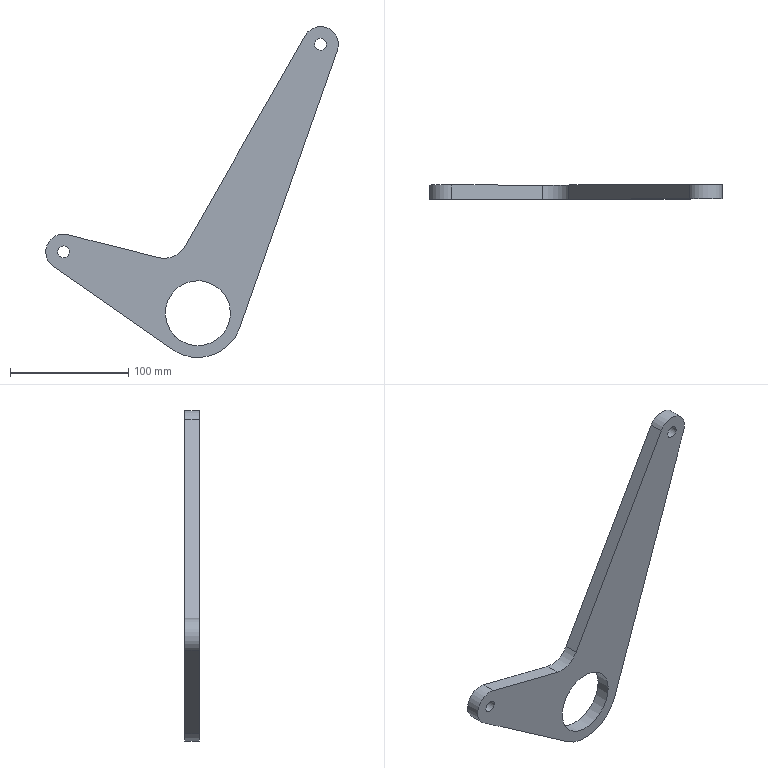Part | NX | features 0 2 | 1 solid | 13 faces | box 247.496 x 12 x 279.945 mm | volume 214925 mm3 | cylinder 7 | plane 6 | commonest cylinder face diameters 10 x2 30 x2 40 x1 55 x1 75 x1
STEP:
#1=CARTESIAN_POINT('',(108.322,86.,-42.76));
#2=VERTEX_POINT('',#1);
#3=CARTESIAN_POINT('',(103.773,86.,-40.685));
#4=DIRECTION('',(0.,-1.,0.));
#5=DIRECTION('',(0.9098,0.,-0.4151));
#6=AXIS2_PLACEMENT_3D('',#3,#4,#5);
#7=CIRCLE('',#6,5.);
#8=EDGE_CURVE('',#2,#2,#7,.T.);
#9=ORIENTED_EDGE('',*,*,#8,.F.);
#10=EDGE_LOOP('',(#9));
#11=FACE_BOUND('',#10,.T.);
#12=CARTESIAN_POINT('',(99.225,74.,-38.609));
#13=VERTEX_POINT('',#12);
#14=CARTESIAN_POINT('',(103.773,74.,-40.685));
#15=DIRECTION('',(0.,1.,0.));
#16=DIRECTION('',(-0.9098,0.,0.4151));
#17=AXIS2_PLACEMENT_3D('',#14,#15,#16);
#18=CIRCLE('',#17,5.);
#19=EDGE_CURVE('',#13,#13,#18,.T.);
#20=ORIENTED_EDGE('',*,*,#19,.F.);
#21=EDGE_LOOP('',(#20));
#22=FACE_BOUND('',#21,.T.);
#23=CARTESIAN_POINT('',(103.773,74.,-40.685));
#24=DIRECTION('',(0.,1.,0.));
#25=DIRECTION('',(-0.9098,0.,0.4151));
#26=AXIS2_PLACEMENT_3D('',#23,#24,#25);
#27=CYLINDRICAL_SURFACE('',#26,5.);
#28=ADVANCED_FACE('',(#11,#22),#27,.F.);
#29=CARTESIAN_POINT('',(-109.173,86.,-218.318));
#30=VERTEX_POINT('',#29);
#31=CARTESIAN_POINT('',(-113.722,86.,-216.243));
#32=DIRECTION('',(0.,-1.,0.));
#33=DIRECTION('',(0.9098,0.,-0.4151));
#34=AXIS2_PLACEMENT_3D('',#31,#32,#33);
#35=CIRCLE('',#34,5.);
#36=EDGE_CURVE('',#30,#30,#35,.T.);
#37=ORIENTED_EDGE('',*,*,#36,.F.);
#38=EDGE_LOOP('',(#37));
#39=FACE_BOUND('',#38,.T.);
#40=CARTESIAN_POINT('',(-118.271,74.,-214.167));
#41=VERTEX_POINT('',#40);
#42=CARTESIAN_POINT('',(-113.722,74.,-216.243));
#43=DIRECTION('',(0.,1.,0.));
#44=DIRECTION('',(-0.9098,0.,0.4151));
#45=AXIS2_PLACEMENT_3D('',#42,#43,#44);
#46=CIRCLE('',#45,5.);
#47=EDGE_CURVE('',#41,#41,#46,.T.);
#48=ORIENTED_EDGE('',*,*,#47,.F.);
#49=EDGE_LOOP('',(#48));
#50=FACE_BOUND('',#49,.T.);
#51=CARTESIAN_POINT('',(-113.722,74.,-216.243));
#52=DIRECTION('',(0.,1.,0.));
#53=DIRECTION('',(-0.9098,0.,0.4151));
#54=AXIS2_PLACEMENT_3D('',#51,#52,#53);
#55=CYLINDRICAL_SURFACE('',#54,5.);
#56=ADVANCED_FACE('',(#39,#50),#55,.F.);
#57=CARTESIAN_POINT('',(35.379,86.,-280.562));
#58=VERTEX_POINT('',#57);
#59=CARTESIAN_POINT('',(35.379,74.,-280.562));
#60=VERTEX_POINT('',#59);
#61=CARTESIAN_POINT('',(35.379,86.,-280.562));
#62=DIRECTION('',(0.,-1.,0.));
#63=VECTOR('',#62,1000.);
#64=LINE('',#61,#63);
#65=EDGE_CURVE('',#58,#60,#64,.T.);
#66=ORIENTED_EDGE('',*,*,#65,.F.);
#67=CARTESIAN_POINT('',(117.925,86.,-45.658));
#68=VERTEX_POINT('',#67);
#69=CARTESIAN_POINT('',(117.925,86.,-45.658));
#70=DIRECTION('',(-0.3315,0.,-0.9434));
#71=VECTOR('',#70,1000.);
#72=LINE('',#69,#71);
#73=EDGE_CURVE('',#68,#58,#72,.T.);
#74=ORIENTED_EDGE('',*,*,#73,.F.);
#75=CARTESIAN_POINT('',(117.925,74.,-45.658));
#76=VERTEX_POINT('',#75);
#77=CARTESIAN_POINT('',(117.925,74.,-45.658));
#78=DIRECTION('',(0.,1.,0.));
#79=VECTOR('',#78,1000.);
#80=LINE('',#77,#79);
#81=EDGE_CURVE('',#76,#68,#80,.T.);
#82=ORIENTED_EDGE('',*,*,#81,.F.);
#83=CARTESIAN_POINT('',(35.379,74.,-280.562));
#84=DIRECTION('',(0.3315,0.,0.9434));
#85=VECTOR('',#84,1000.);
#86=LINE('',#83,#85);
#87=EDGE_CURVE('',#60,#76,#86,.T.);
#88=ORIENTED_EDGE('',*,*,#87,.F.);
#89=EDGE_LOOP('',(#66,#74,#82,#88));
#90=FACE_BOUND('',#89,.T.);
#91=CARTESIAN_POINT('',(117.925,86.,-45.658));
#92=DIRECTION('',(-0.9434,0.,0.3315));
#93=DIRECTION('',(0.3315,0.,0.9434));
#94=AXIS2_PLACEMENT_3D('',#91,#92,#93);
#95=PLANE('',#94);
#96=ADVANCED_FACE('',(#90),#95,.F.);
#97=CARTESIAN_POINT('',(-21.453,86.,-298.887));
#98=VERTEX_POINT('',#97);
#99=CARTESIAN_POINT('',(0.,86.,-268.129));
#100=DIRECTION('',(0.,1.,0.));
#101=DIRECTION('',(0.9098,0.,-0.4151));
#102=AXIS2_PLACEMENT_3D('',#99,#100,#101);
#103=CIRCLE('',#102,37.5);
#104=EDGE_CURVE('',#58,#98,#103,.T.);
#105=ORIENTED_EDGE('',*,*,#104,.F.);
#106=ORIENTED_EDGE('',*,*,#65,.T.);
#107=CARTESIAN_POINT('',(-21.453,74.,-298.887));
#108=VERTEX_POINT('',#107);
#109=CARTESIAN_POINT('',(0.,74.,-268.129));
#110=DIRECTION('',(0.,-1.,0.));
#111=DIRECTION('',(0.9098,0.,-0.4151));
#112=AXIS2_PLACEMENT_3D('',#109,#110,#111);
#113=CIRCLE('',#112,37.5);
#114=EDGE_CURVE('',#108,#60,#113,.T.);
#115=ORIENTED_EDGE('',*,*,#114,.F.);
#116=CARTESIAN_POINT('',(-21.453,74.,-298.887));
#117=DIRECTION('',(0.,1.,0.));
#118=VECTOR('',#117,1000.);
#119=LINE('',#116,#118);
#120=EDGE_CURVE('',#108,#98,#119,.T.);
#121=ORIENTED_EDGE('',*,*,#120,.T.);
#122=EDGE_LOOP('',(#105,#106,#115,#121));
#123=FACE_BOUND('',#122,.T.);
#124=CARTESIAN_POINT('',(0.,86.,-268.129));
#125=DIRECTION('',(0.,-1.,0.));
#126=DIRECTION('',(0.9098,0.,-0.4151));
#127=AXIS2_PLACEMENT_3D('',#124,#125,#126);
#128=CYLINDRICAL_SURFACE('',#127,37.5);
#129=ADVANCED_FACE('',(#123),#128,.T.);
#130=CARTESIAN_POINT('',(-122.303,86.,-228.546));
#131=VERTEX_POINT('',#130);
#132=CARTESIAN_POINT('',(-122.303,74.,-228.546));
#133=VERTEX_POINT('',#132);
#134=CARTESIAN_POINT('',(-122.303,86.,-228.546));
#135=DIRECTION('',(0.,-1.,0.));
#136=VECTOR('',#135,1000.);
#137=LINE('',#134,#136);
#138=EDGE_CURVE('',#131,#133,#137,.T.);
#139=ORIENTED_EDGE('',*,*,#138,.F.);
#140=CARTESIAN_POINT('',(-21.453,86.,-298.887));
#141=DIRECTION('',(-0.8202,0.,0.5721));
#142=VECTOR('',#141,1000.);
#143=LINE('',#140,#142);
#144=EDGE_CURVE('',#98,#131,#143,.T.);
#145=ORIENTED_EDGE('',*,*,#144,.F.);
#146=ORIENTED_EDGE('',*,*,#120,.F.);
#147=CARTESIAN_POINT('',(-122.303,74.,-228.546));
#148=DIRECTION('',(0.8202,0.,-0.5721));
#149=VECTOR('',#148,1000.);
#150=LINE('',#147,#149);
#151=EDGE_CURVE('',#133,#108,#150,.T.);
#152=ORIENTED_EDGE('',*,*,#151,.F.);
#153=EDGE_LOOP('',(#139,#145,#146,#152));
#154=FACE_BOUND('',#153,.T.);
#155=CARTESIAN_POINT('',(-21.453,86.,-298.887));
#156=DIRECTION('',(0.5721,0.,0.8202));
#157=DIRECTION('',(0.8202,0.,-0.5721));
#158=AXIS2_PLACEMENT_3D('',#155,#156,#157);
#159=PLANE('',#158);
#160=ADVANCED_FACE('',(#154),#159,.F.);
#161=CARTESIAN_POINT('',(-110.054,74.,-201.698));
#162=VERTEX_POINT('',#161);
#163=CARTESIAN_POINT('',(-110.054,86.,-201.698));
#164=VERTEX_POINT('',#163);
#165=CARTESIAN_POINT('',(-110.054,74.,-201.698));
#166=DIRECTION('',(0.,1.,0.));
#167=VECTOR('',#166,1000.);
#168=LINE('',#165,#167);
#169=EDGE_CURVE('',#162,#164,#168,.T.);
#170=ORIENTED_EDGE('',*,*,#169,.T.);
#171=CARTESIAN_POINT('',(-113.722,86.,-216.243));
#172=DIRECTION('',(0.,1.,0.));
#173=DIRECTION('',(-0.5721,0.,-0.8202));
#174=AXIS2_PLACEMENT_3D('',#171,#172,#173);
#175=CIRCLE('',#174,15.);
#176=EDGE_CURVE('',#131,#164,#175,.T.);
#177=ORIENTED_EDGE('',*,*,#176,.F.);
#178=ORIENTED_EDGE('',*,*,#138,.T.);
#179=CARTESIAN_POINT('',(-113.722,74.,-216.243));
#180=DIRECTION('',(0.,-1.,0.));
#181=DIRECTION('',(0.2446,0.,0.9696));
#182=AXIS2_PLACEMENT_3D('',#179,#180,#181);
#183=CIRCLE('',#182,15.);
#184=EDGE_CURVE('',#162,#133,#183,.T.);
#185=ORIENTED_EDGE('',*,*,#184,.F.);
#186=EDGE_LOOP('',(#170,#177,#178,#185));
#187=FACE_BOUND('',#186,.T.);
#188=CARTESIAN_POINT('',(-113.722,86.,-216.243));
#189=DIRECTION('',(0.,-1.,0.));
#190=DIRECTION('',(0.9098,0.,-0.4151));
#191=AXIS2_PLACEMENT_3D('',#188,#189,#190);
#192=CYLINDRICAL_SURFACE('',#191,15.);
#193=ADVANCED_FACE('',(#187),#192,.T.);
#194=CARTESIAN_POINT('',(-33.2,86.,-221.082));
#195=VERTEX_POINT('',#194);
#196=CARTESIAN_POINT('',(-33.2,74.,-221.082));
#197=VERTEX_POINT('',#196);
#198=CARTESIAN_POINT('',(-33.2,86.,-221.082));
#199=DIRECTION('',(0.,-1.,0.));
#200=VECTOR('',#199,1000.);
#201=LINE('',#198,#200);
#202=EDGE_CURVE('',#195,#197,#201,.T.);
#203=ORIENTED_EDGE('',*,*,#202,.F.);
#204=CARTESIAN_POINT('',(-110.054,86.,-201.698));
#205=DIRECTION('',(0.9696,0.,-0.2446));
#206=VECTOR('',#205,1000.);
#207=LINE('',#204,#206);
#208=EDGE_CURVE('',#164,#195,#207,.T.);
#209=ORIENTED_EDGE('',*,*,#208,.F.);
#210=ORIENTED_EDGE('',*,*,#169,.F.);
#211=CARTESIAN_POINT('',(-33.2,74.,-221.082));
#212=DIRECTION('',(-0.9696,0.,0.2446));
#213=VECTOR('',#212,1000.);
#214=LINE('',#211,#213);
#215=EDGE_CURVE('',#197,#162,#214,.T.);
#216=ORIENTED_EDGE('',*,*,#215,.F.);
#217=EDGE_LOOP('',(#203,#209,#210,#216));
#218=FACE_BOUND('',#217,.T.);
#219=CARTESIAN_POINT('',(-110.054,86.,-201.698));
#220=DIRECTION('',(-0.2446,0.,-0.9696));
#221=DIRECTION('',(-0.9696,0.,0.2446));
#222=AXIS2_PLACEMENT_3D('',#219,#220,#221);
#223=PLANE('',#222);
#224=ADVANCED_FACE('',(#218),#223,.F.);
#225=ORIENTED_EDGE('',*,*,#202,.T.);
#226=CARTESIAN_POINT('',(-10.934,74.,-211.595));
#227=VERTEX_POINT('',#226);
#228=CARTESIAN_POINT('',(-28.309,74.,-201.689));
#229=DIRECTION('',(0.,1.,0.));
#230=DIRECTION('',(0.8687,0.,-0.4953));
#231=AXIS2_PLACEMENT_3D('',#228,#229,#230);
#232=CIRCLE('',#231,20.);
#233=EDGE_CURVE('',#227,#197,#232,.T.);
#234=ORIENTED_EDGE('',*,*,#233,.F.);
#235=CARTESIAN_POINT('',(-10.934,86.,-211.595));
#236=VERTEX_POINT('',#235);
#237=CARTESIAN_POINT('',(-10.934,74.,-211.595));
#238=DIRECTION('',(0.,1.,0.));
#239=VECTOR('',#238,1000.);
#240=LINE('',#237,#239);
#241=EDGE_CURVE('',#227,#236,#240,.T.);
#242=ORIENTED_EDGE('',*,*,#241,.T.);
#243=CARTESIAN_POINT('',(-28.309,86.,-201.689));
#244=DIRECTION('',(0.,-1.,0.));
#245=DIRECTION('',(-0.2446,0.,-0.9696));
#246=AXIS2_PLACEMENT_3D('',#243,#244,#245);
#247=CIRCLE('',#246,20.);
#248=EDGE_CURVE('',#195,#236,#247,.T.);
#249=ORIENTED_EDGE('',*,*,#248,.F.);
#250=EDGE_LOOP('',(#225,#234,#242,#249));
#251=FACE_BOUND('',#250,.T.);
#252=CARTESIAN_POINT('',(-28.309,86.,-201.689));
#253=DIRECTION('',(0.,1.,0.));
#254=DIRECTION('',(-0.9098,0.,0.4151));
#255=AXIS2_PLACEMENT_3D('',#252,#253,#254);
#256=CYLINDRICAL_SURFACE('',#255,20.);
#257=ADVANCED_FACE('',(#251),#256,.F.);
#258=ORIENTED_EDGE('',*,*,#8,.T.);
#259=EDGE_LOOP('',(#258));
#260=FACE_BOUND('',#259,.T.);
#261=ORIENTED_EDGE('',*,*,#36,.T.);
#262=EDGE_LOOP('',(#261));
#263=FACE_BOUND('',#262,.T.);
#264=CARTESIAN_POINT('',(-25.019,86.,-256.714));
#265=VERTEX_POINT('',#264);
#266=CARTESIAN_POINT('',(0.,86.,-268.129));
#267=DIRECTION('',(0.,-1.,0.));
#268=DIRECTION('',(-0.9098,0.,0.4151));
#269=AXIS2_PLACEMENT_3D('',#266,#267,#268);
#270=CIRCLE('',#269,27.5);
#271=EDGE_CURVE('',#265,#265,#270,.T.);
#272=ORIENTED_EDGE('',*,*,#271,.T.);
#273=EDGE_LOOP('',(#272));
#274=FACE_BOUND('',#273,.T.);
#275=ORIENTED_EDGE('',*,*,#73,.T.);
#276=ORIENTED_EDGE('',*,*,#104,.T.);
#277=ORIENTED_EDGE('',*,*,#144,.T.);
#278=ORIENTED_EDGE('',*,*,#176,.T.);
#279=ORIENTED_EDGE('',*,*,#208,.T.);
#280=ORIENTED_EDGE('',*,*,#248,.T.);
#281=CARTESIAN_POINT('',(90.743,86.,-33.255));
#282=VERTEX_POINT('',#281);
#283=CARTESIAN_POINT('',(-10.934,86.,-211.595));
#284=DIRECTION('',(0.4953,0.,0.8687));
#285=VECTOR('',#284,1000.);
#286=LINE('',#283,#285);
#287=EDGE_CURVE('',#236,#282,#286,.T.);
#288=ORIENTED_EDGE('',*,*,#287,.T.);
#289=CARTESIAN_POINT('',(103.773,86.,-40.685));
#290=DIRECTION('',(0.,1.,0.));
#291=DIRECTION('',(-0.8687,0.,0.4953));
#292=AXIS2_PLACEMENT_3D('',#289,#290,#291);
#293=CIRCLE('',#292,15.);
#294=EDGE_CURVE('',#282,#68,#293,.T.);
#295=ORIENTED_EDGE('',*,*,#294,.T.);
#296=EDGE_LOOP('',(#275,#276,#277,#278,#279,#280,#288,#295));
#297=FACE_BOUND('',#296,.T.);
#298=CARTESIAN_POINT('',(103.773,86.,-40.685));
#299=DIRECTION('',(0.,1.,0.));
#300=DIRECTION('',(-0.9098,0.,0.4151));
#301=AXIS2_PLACEMENT_3D('',#298,#299,#300);
#302=PLANE('',#301);
#303=ADVANCED_FACE('',(#260,#263,#274,#297),#302,.T.);
#304=ORIENTED_EDGE('',*,*,#241,.F.);
#305=CARTESIAN_POINT('',(90.743,74.,-33.255));
#306=VERTEX_POINT('',#305);
#307=CARTESIAN_POINT('',(90.743,74.,-33.255));
#308=DIRECTION('',(-0.4953,0.,-0.8687));
#309=VECTOR('',#308,1000.);
#310=LINE('',#307,#309);
#311=EDGE_CURVE('',#306,#227,#310,.T.);
#312=ORIENTED_EDGE('',*,*,#311,.F.);
#313=CARTESIAN_POINT('',(90.743,86.,-33.255));
#314=DIRECTION('',(0.,-1.,0.));
#315=VECTOR('',#314,1000.);
#316=LINE('',#313,#315);
#317=EDGE_CURVE('',#282,#306,#316,.T.);
#318=ORIENTED_EDGE('',*,*,#317,.F.);
#319=ORIENTED_EDGE('',*,*,#287,.F.);
#320=EDGE_LOOP('',(#304,#312,#318,#319));
#321=FACE_BOUND('',#320,.T.);
#322=CARTESIAN_POINT('',(90.743,86.,-33.255));
#323=DIRECTION('',(0.8687,0.,-0.4953));
#324=DIRECTION('',(-0.4953,0.,-0.8687));
#325=AXIS2_PLACEMENT_3D('',#322,#323,#324);
#326=PLANE('',#325);
#327=ADVANCED_FACE('',(#321),#326,.F.);
#328=ORIENTED_EDGE('',*,*,#81,.T.);
#329=ORIENTED_EDGE('',*,*,#294,.F.);
#330=ORIENTED_EDGE('',*,*,#317,.T.);
#331=CARTESIAN_POINT('',(103.773,74.,-40.685));
#332=DIRECTION('',(0.,-1.,0.));
#333=DIRECTION('',(0.9434,0.,-0.3315));
#334=AXIS2_PLACEMENT_3D('',#331,#332,#333);
#335=CIRCLE('',#334,15.);
#336=EDGE_CURVE('',#76,#306,#335,.T.);
#337=ORIENTED_EDGE('',*,*,#336,.F.);
#338=EDGE_LOOP('',(#328,#329,#330,#337));
#339=FACE_BOUND('',#338,.T.);
#340=CARTESIAN_POINT('',(103.773,86.,-40.685));
#341=DIRECTION('',(0.,-1.,0.));
#342=DIRECTION('',(0.9098,0.,-0.4151));
#343=AXIS2_PLACEMENT_3D('',#340,#341,#342);
#344=CYLINDRICAL_SURFACE('',#343,15.);
#345=ADVANCED_FACE('',(#339),#344,.T.);
#346=ORIENTED_EDGE('',*,*,#19,.T.);
#347=EDGE_LOOP('',(#346));
#348=FACE_BOUND('',#347,.T.);
#349=ORIENTED_EDGE('',*,*,#47,.T.);
#350=EDGE_LOOP('',(#349));
#351=FACE_BOUND('',#350,.T.);
#352=CARTESIAN_POINT('',(25.019,74.,-279.545));
#353=VERTEX_POINT('',#352);
#354=CARTESIAN_POINT('',(0.,74.,-268.129));
#355=DIRECTION('',(0.,1.,0.));
#356=DIRECTION('',(0.9098,0.,-0.4151));
#357=AXIS2_PLACEMENT_3D('',#354,#355,#356);
#358=CIRCLE('',#357,27.5);
#359=EDGE_CURVE('',#353,#353,#358,.T.);
#360=ORIENTED_EDGE('',*,*,#359,.T.);
#361=EDGE_LOOP('',(#360));
#362=FACE_BOUND('',#361,.T.);
#363=ORIENTED_EDGE('',*,*,#311,.T.);
#364=ORIENTED_EDGE('',*,*,#233,.T.);
#365=ORIENTED_EDGE('',*,*,#215,.T.);
#366=ORIENTED_EDGE('',*,*,#184,.T.);
#367=ORIENTED_EDGE('',*,*,#151,.T.);
#368=ORIENTED_EDGE('',*,*,#114,.T.);
#369=ORIENTED_EDGE('',*,*,#87,.T.);
#370=ORIENTED_EDGE('',*,*,#336,.T.);
#371=EDGE_LOOP('',(#363,#364,#365,#366,#367,#368,#369,#370));
#372=FACE_BOUND('',#371,.T.);
#373=CARTESIAN_POINT('',(103.773,74.,-40.685));
#374=DIRECTION('',(0.,1.,0.));
#375=DIRECTION('',(-0.9098,0.,0.4151));
#376=AXIS2_PLACEMENT_3D('',#373,#374,#375);
#377=PLANE('',#376);
#378=ADVANCED_FACE('',(#348,#351,#362,#372),#377,.F.);
#379=ORIENTED_EDGE('',*,*,#271,.F.);
#380=EDGE_LOOP('',(#379));
#381=FACE_BOUND('',#380,.T.);
#382=ORIENTED_EDGE('',*,*,#359,.F.);
#383=EDGE_LOOP('',(#382));
#384=FACE_BOUND('',#383,.T.);
#385=CARTESIAN_POINT('',(0.,74.,-268.129));
#386=DIRECTION('',(0.,1.,0.));
#387=DIRECTION('',(-0.9098,0.,0.4151));
#388=AXIS2_PLACEMENT_3D('',#385,#386,#387);
#389=CYLINDRICAL_SURFACE('',#388,27.5);
#390=ADVANCED_FACE('',(#381,#384),#389,.F.);
#391=CLOSED_SHELL('',(#28,#56,#96,#129,#160,#193,#224,#257,#303,#327,#345,#378,#390));
#392=MANIFOLD_SOLID_BREP('',#391);
#393=(LENGTH_UNIT()NAMED_UNIT(*)SI_UNIT(.MILLI.,.METRE.));
#394=UNCERTAINTY_MEASURE_WITH_UNIT(LENGTH_MEASURE(0.00001),#393,'','');
#395=(NAMED_UNIT(*)PLANE_ANGLE_UNIT()SI_UNIT($,.RADIAN.));
#396=(NAMED_UNIT(*)SI_UNIT($,.STERADIAN.)SOLID_ANGLE_UNIT());
#397=(GEOMETRIC_REPRESENTATION_CONTEXT(3)GLOBAL_UNCERTAINTY_ASSIGNED_CONTEXT((#394))GLOBAL_UNIT_ASSIGNED_CONTEXT((#393,#395,#396))REPRESENTATION_CONTEXT('',''));
#398=ADVANCED_BREP_SHAPE_REPRESENTATION('',(#392),#397);